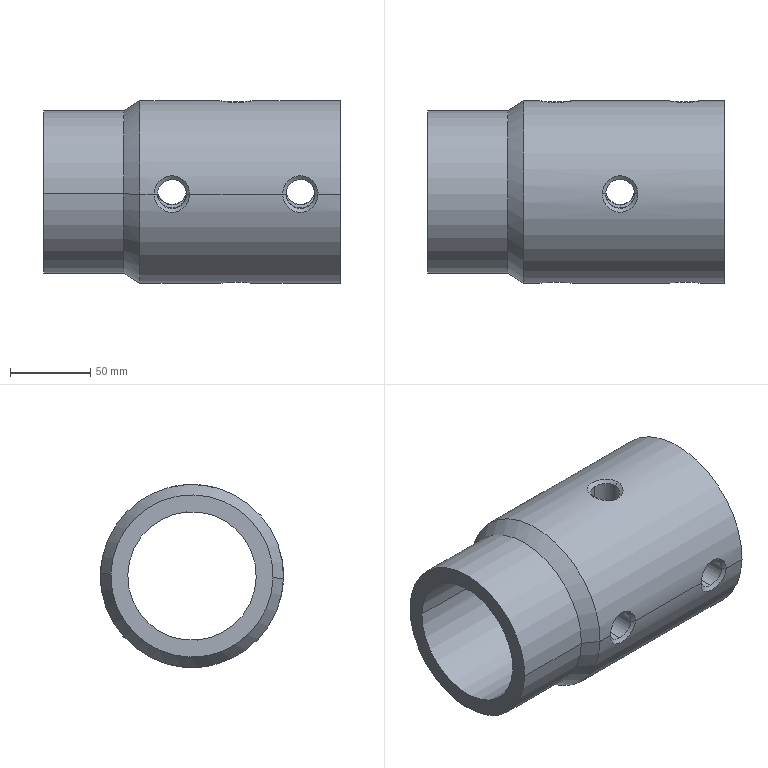Part | STEP file | Input 124 | 1 solid | 36 faces | box 185 x 114 x 114 mm | volume 807255 mm3 | cylinder 18 | spline 12 | cone 4 | plane 2 | commonest cylinder face diameters 18 x12 80 x2 101 x2 114 x2